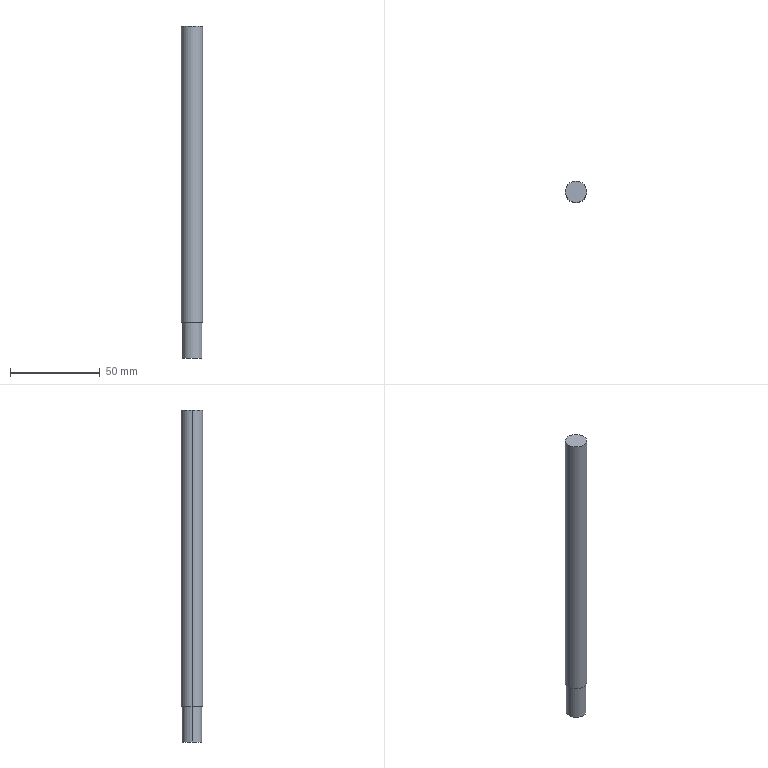Part | SolidWorks | features MirrorStock 1 | 1 solid | 7 faces | box 12 x 12 x 185 mm | volume 20562 mm3 | cylinder 4 | plane 3 | commonest cylinder face diameters 11 x2 12 x2
STEP:
#1=CARTESIAN_POINT('',(-5.5,0.,-72.5));
#2=VERTEX_POINT('',#1);
#3=CARTESIAN_POINT('',(5.5,0.,-72.5));
#4=VERTEX_POINT('',#3);
#5=CARTESIAN_POINT('',(0.,0.,-72.5));
#6=DIRECTION('',(0.,0.,1.));
#7=DIRECTION('',(1.,0.,0.));
#8=AXIS2_PLACEMENT_3D('',#5,#6,#7);
#9=CIRCLE('',#8,5.5);
#10=EDGE_CURVE('',#2,#4,#9,.T.);
#11=ORIENTED_EDGE('',*,*,#10,.F.);
#12=CARTESIAN_POINT('',(-5.5,0.,-92.5));
#13=VERTEX_POINT('',#12);
#14=CARTESIAN_POINT('',(-5.5,0.,-72.5));
#15=DIRECTION('',(0.,0.,-1.));
#16=VECTOR('',#15,1000.);
#17=LINE('',#14,#16);
#18=EDGE_CURVE('',#2,#13,#17,.T.);
#19=ORIENTED_EDGE('',*,*,#18,.T.);
#20=CARTESIAN_POINT('',(5.5,0.,-92.5));
#21=VERTEX_POINT('',#20);
#22=CARTESIAN_POINT('',(0.,0.,-92.5));
#23=DIRECTION('',(0.,0.,1.));
#24=DIRECTION('',(1.,0.,0.));
#25=AXIS2_PLACEMENT_3D('',#22,#23,#24);
#26=CIRCLE('',#25,5.5);
#27=EDGE_CURVE('',#13,#21,#26,.T.);
#28=ORIENTED_EDGE('',*,*,#27,.T.);
#29=CARTESIAN_POINT('',(5.5,0.,-72.5));
#30=DIRECTION('',(0.,0.,-1.));
#31=VECTOR('',#30,1000.);
#32=LINE('',#29,#31);
#33=EDGE_CURVE('',#4,#21,#32,.T.);
#34=ORIENTED_EDGE('',*,*,#33,.F.);
#35=EDGE_LOOP('',(#11,#19,#28,#34));
#36=FACE_OUTER_BOUND('',#35,.T.);
#37=CARTESIAN_POINT('',(0.,0.,-72.5));
#38=DIRECTION('',(0.,0.,-1.));
#39=DIRECTION('',(1.,0.,0.));
#40=AXIS2_PLACEMENT_3D('',#37,#38,#39);
#41=CYLINDRICAL_SURFACE('',#40,5.5);
#42=ADVANCED_FACE('',(#36),#41,.T.);
#43=CARTESIAN_POINT('',(-6.,0.,-72.5));
#44=VERTEX_POINT('',#43);
#45=CARTESIAN_POINT('',(6.,0.,-72.5));
#46=VERTEX_POINT('',#45);
#47=CARTESIAN_POINT('',(0.,0.,-72.5));
#48=DIRECTION('',(0.,0.,1.));
#49=DIRECTION('',(1.,0.,0.));
#50=AXIS2_PLACEMENT_3D('',#47,#48,#49);
#51=CIRCLE('',#50,6.);
#52=EDGE_CURVE('',#44,#46,#51,.T.);
#53=ORIENTED_EDGE('',*,*,#52,.T.);
#54=CARTESIAN_POINT('',(6.,0.,92.5));
#55=VERTEX_POINT('',#54);
#56=CARTESIAN_POINT('',(6.,0.,-92.5));
#57=DIRECTION('',(0.,0.,1.));
#58=VECTOR('',#57,1000.);
#59=LINE('',#56,#58);
#60=EDGE_CURVE('',#46,#55,#59,.T.);
#61=ORIENTED_EDGE('',*,*,#60,.T.);
#62=CARTESIAN_POINT('',(-6.,0.,92.5));
#63=VERTEX_POINT('',#62);
#64=CARTESIAN_POINT('',(0.,0.,92.5));
#65=DIRECTION('',(0.,0.,1.));
#66=DIRECTION('',(1.,0.,0.));
#67=AXIS2_PLACEMENT_3D('',#64,#65,#66);
#68=CIRCLE('',#67,6.);
#69=EDGE_CURVE('',#63,#55,#68,.T.);
#70=ORIENTED_EDGE('',*,*,#69,.F.);
#71=CARTESIAN_POINT('',(-6.,0.,-92.5));
#72=DIRECTION('',(0.,0.,1.));
#73=VECTOR('',#72,1000.);
#74=LINE('',#71,#73);
#75=EDGE_CURVE('',#44,#63,#74,.T.);
#76=ORIENTED_EDGE('',*,*,#75,.F.);
#77=EDGE_LOOP('',(#53,#61,#70,#76));
#78=FACE_OUTER_BOUND('',#77,.T.);
#79=CARTESIAN_POINT('',(0.,0.,-92.5));
#80=DIRECTION('',(0.,0.,1.));
#81=DIRECTION('',(-1.,0.,0.));
#82=AXIS2_PLACEMENT_3D('',#79,#80,#81);
#83=CYLINDRICAL_SURFACE('',#82,6.);
#84=ADVANCED_FACE('',(#78),#83,.T.);
#85=ORIENTED_EDGE('',*,*,#60,.F.);
#86=CARTESIAN_POINT('',(0.,0.,-72.5));
#87=DIRECTION('',(0.,0.,1.));
#88=DIRECTION('',(1.,0.,0.));
#89=AXIS2_PLACEMENT_3D('',#86,#87,#88);
#90=CIRCLE('',#89,6.);
#91=EDGE_CURVE('',#46,#44,#90,.T.);
#92=ORIENTED_EDGE('',*,*,#91,.T.);
#93=ORIENTED_EDGE('',*,*,#75,.T.);
#94=CARTESIAN_POINT('',(0.,0.,92.5));
#95=DIRECTION('',(0.,0.,1.));
#96=DIRECTION('',(1.,0.,0.));
#97=AXIS2_PLACEMENT_3D('',#94,#95,#96);
#98=CIRCLE('',#97,6.);
#99=EDGE_CURVE('',#55,#63,#98,.T.);
#100=ORIENTED_EDGE('',*,*,#99,.F.);
#101=EDGE_LOOP('',(#85,#92,#93,#100));
#102=FACE_OUTER_BOUND('',#101,.T.);
#103=CARTESIAN_POINT('',(0.,0.,-92.5));
#104=DIRECTION('',(0.,0.,1.));
#105=DIRECTION('',(-1.,0.,0.));
#106=AXIS2_PLACEMENT_3D('',#103,#104,#105);
#107=CYLINDRICAL_SURFACE('',#106,6.);
#108=ADVANCED_FACE('',(#102),#107,.T.);
#109=ORIENTED_EDGE('',*,*,#69,.T.);
#110=ORIENTED_EDGE('',*,*,#99,.T.);
#111=EDGE_LOOP('',(#109,#110));
#112=FACE_OUTER_BOUND('',#111,.T.);
#113=CARTESIAN_POINT('',(0.,0.,92.5));
#114=DIRECTION('',(0.,0.,-1.));
#115=DIRECTION('',(1.,0.,0.));
#116=AXIS2_PLACEMENT_3D('',#113,#114,#115);
#117=PLANE('',#116);
#118=ADVANCED_FACE('',(#112),#117,.F.);
#119=CARTESIAN_POINT('',(0.,0.,-72.5));
#120=DIRECTION('',(0.,0.,1.));
#121=DIRECTION('',(1.,0.,0.));
#122=AXIS2_PLACEMENT_3D('',#119,#120,#121);
#123=CIRCLE('',#122,5.5);
#124=EDGE_CURVE('',#4,#2,#123,.T.);
#125=ORIENTED_EDGE('',*,*,#124,.T.);
#126=ORIENTED_EDGE('',*,*,#10,.T.);
#127=EDGE_LOOP('',(#125,#126));
#128=FACE_BOUND('',#127,.T.);
#129=ORIENTED_EDGE('',*,*,#52,.F.);
#130=ORIENTED_EDGE('',*,*,#91,.F.);
#131=EDGE_LOOP('',(#129,#130));
#132=FACE_OUTER_BOUND('',#131,.T.);
#133=CARTESIAN_POINT('',(0.,0.,-72.5));
#134=DIRECTION('',(0.,0.,-1.));
#135=DIRECTION('',(1.,0.,0.));
#136=AXIS2_PLACEMENT_3D('',#133,#134,#135);
#137=PLANE('',#136);
#138=ADVANCED_FACE('',(#128,#132),#137,.T.);
#139=ORIENTED_EDGE('',*,*,#18,.F.);
#140=ORIENTED_EDGE('',*,*,#124,.F.);
#141=ORIENTED_EDGE('',*,*,#33,.T.);
#142=CARTESIAN_POINT('',(0.,0.,-92.5));
#143=DIRECTION('',(0.,0.,1.));
#144=DIRECTION('',(1.,0.,0.));
#145=AXIS2_PLACEMENT_3D('',#142,#143,#144);
#146=CIRCLE('',#145,5.5);
#147=EDGE_CURVE('',#21,#13,#146,.T.);
#148=ORIENTED_EDGE('',*,*,#147,.T.);
#149=EDGE_LOOP('',(#139,#140,#141,#148));
#150=FACE_OUTER_BOUND('',#149,.T.);
#151=CARTESIAN_POINT('',(0.,0.,-72.5));
#152=DIRECTION('',(0.,0.,-1.));
#153=DIRECTION('',(1.,0.,0.));
#154=AXIS2_PLACEMENT_3D('',#151,#152,#153);
#155=CYLINDRICAL_SURFACE('',#154,5.5);
#156=ADVANCED_FACE('',(#150),#155,.T.);
#157=ORIENTED_EDGE('',*,*,#147,.F.);
#158=ORIENTED_EDGE('',*,*,#27,.F.);
#159=EDGE_LOOP('',(#157,#158));
#160=FACE_OUTER_BOUND('',#159,.T.);
#161=CARTESIAN_POINT('',(0.,0.,-92.5));
#162=DIRECTION('',(0.,0.,-1.));
#163=DIRECTION('',(1.,0.,0.));
#164=AXIS2_PLACEMENT_3D('',#161,#162,#163);
#165=PLANE('',#164);
#166=ADVANCED_FACE('',(#160),#165,.T.);
#167=CLOSED_SHELL('',(#42,#84,#108,#118,#138,#156,#166));
#168=MANIFOLD_SOLID_BREP('',#167);
#169=CARTESIAN_POINT('',(0.,0.,0.));
#170=DIRECTION('',(0.,0.,1.));
#171=DIRECTION('',(1.,0.,0.));
#172=AXIS2_PLACEMENT_3D('',#169,#170,#171);
#173=(LENGTH_UNIT()NAMED_UNIT(*)SI_UNIT(.MILLI.,.METRE.));
#174=UNCERTAINTY_MEASURE_WITH_UNIT(LENGTH_MEASURE(0.00001),#173,'','');
#175=(NAMED_UNIT(*)PLANE_ANGLE_UNIT()SI_UNIT($,.RADIAN.));
#176=(NAMED_UNIT(*)SI_UNIT($,.STERADIAN.)SOLID_ANGLE_UNIT());
#177=(GEOMETRIC_REPRESENTATION_CONTEXT(3)GLOBAL_UNCERTAINTY_ASSIGNED_CONTEXT((#174))GLOBAL_UNIT_ASSIGNED_CONTEXT((#173,#175,#176))REPRESENTATION_CONTEXT('',''));
#178=ADVANCED_BREP_SHAPE_REPRESENTATION('',(#168,#172),#177);